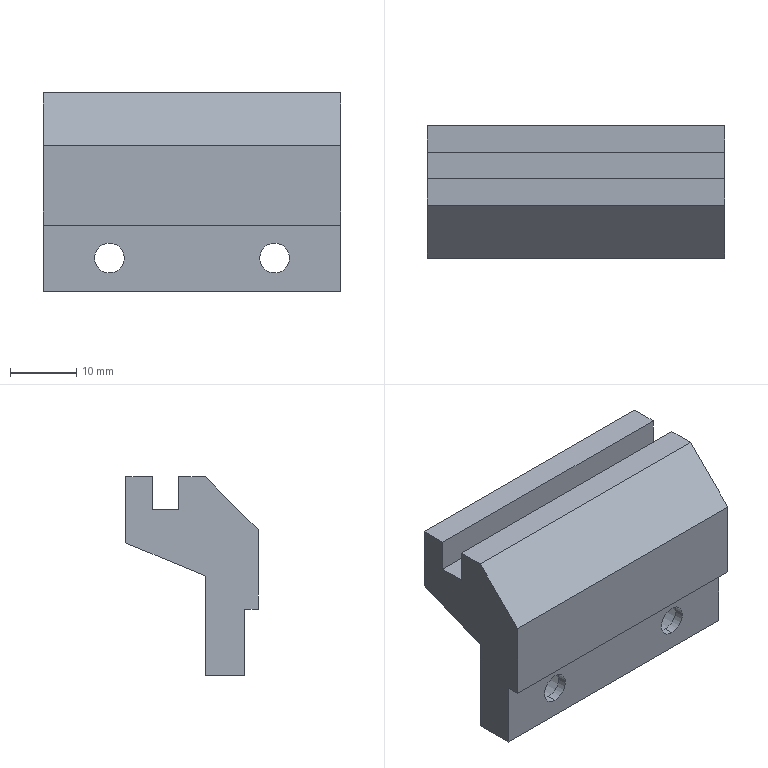Part | SolidWorks | features ICE 2, Chamfer 1, Extrusion 1, HoleWzd 1 | 1 solid | 25 faces | box 45 x 20 x 30 mm | volume 13803 mm3 | plane 17 | cylinder 8 | commonest cylinder face diameters 4.5 x4 8 x4
STEP:
#1=CARTESIAN_POINT('',(-12.5,-6.6,1.));
#2=VERTEX_POINT('',#1);
#3=CARTESIAN_POINT('',(-12.5,-6.6,9.));
#4=VERTEX_POINT('',#3);
#5=CARTESIAN_POINT('',(-12.5,-6.6,5.));
#6=DIRECTION('',(0.,1.,0.));
#7=DIRECTION('',(0.,0.,1.));
#8=AXIS2_PLACEMENT_3D('',#5,#6,#7);
#9=CIRCLE('',#8,4.);
#10=EDGE_CURVE('',#2,#4,#9,.T.);
#11=ORIENTED_EDGE('',*,*,#10,.F.);
#12=CARTESIAN_POINT('',(-12.5,-2.,1.));
#13=VERTEX_POINT('',#12);
#14=CARTESIAN_POINT('',(-12.5,-2.,1.));
#15=DIRECTION('',(0.,1.,0.));
#16=VECTOR('',#15,1000.);
#17=LINE('',#14,#16);
#18=EDGE_CURVE('',#2,#13,#17,.T.);
#19=ORIENTED_EDGE('',*,*,#18,.T.);
#20=CARTESIAN_POINT('',(-12.5,-2.,9.));
#21=VERTEX_POINT('',#20);
#22=CARTESIAN_POINT('',(-12.5,-2.,5.));
#23=DIRECTION('',(0.,1.,0.));
#24=DIRECTION('',(0.,0.,1.));
#25=AXIS2_PLACEMENT_3D('',#22,#23,#24);
#26=CIRCLE('',#25,4.);
#27=EDGE_CURVE('',#13,#21,#26,.T.);
#28=ORIENTED_EDGE('',*,*,#27,.T.);
#29=CARTESIAN_POINT('',(-12.5,-2.,9.));
#30=DIRECTION('',(0.,1.,0.));
#31=VECTOR('',#30,1000.);
#32=LINE('',#29,#31);
#33=EDGE_CURVE('',#4,#21,#32,.T.);
#34=ORIENTED_EDGE('',*,*,#33,.F.);
#35=EDGE_LOOP('',(#11,#19,#28,#34));
#36=FACE_OUTER_BOUND('',#35,.T.);
#37=CARTESIAN_POINT('',(-12.5,-2.,5.));
#38=DIRECTION('',(0.,1.,0.));
#39=DIRECTION('',(0.,0.,1.));
#40=AXIS2_PLACEMENT_3D('',#37,#38,#39);
#41=CYLINDRICAL_SURFACE('',#40,4.);
#42=ADVANCED_FACE('',(#36),#41,.F.);
#43=CARTESIAN_POINT('',(-12.5,-8.,7.25));
#44=VERTEX_POINT('',#43);
#45=CARTESIAN_POINT('',(-12.5,-8.,2.75));
#46=VERTEX_POINT('',#45);
#47=CARTESIAN_POINT('',(-12.5,-8.,5.));
#48=DIRECTION('',(0.,-1.,0.));
#49=DIRECTION('',(0.,0.,1.));
#50=AXIS2_PLACEMENT_3D('',#47,#48,#49);
#51=CIRCLE('',#50,2.25);
#52=EDGE_CURVE('',#44,#46,#51,.T.);
#53=ORIENTED_EDGE('',*,*,#52,.T.);
#54=CARTESIAN_POINT('',(-12.5,-6.6,2.75));
#55=VERTEX_POINT('',#54);
#56=CARTESIAN_POINT('',(-12.5,-2.,2.75));
#57=DIRECTION('',(0.,1.,0.));
#58=VECTOR('',#57,1000.);
#59=LINE('',#56,#58);
#60=EDGE_CURVE('',#46,#55,#59,.T.);
#61=ORIENTED_EDGE('',*,*,#60,.T.);
#62=CARTESIAN_POINT('',(-12.5,-6.6,7.25));
#63=VERTEX_POINT('',#62);
#64=CARTESIAN_POINT('',(-12.5,-6.6,5.));
#65=DIRECTION('',(0.,1.,0.));
#66=DIRECTION('',(0.,0.,1.));
#67=AXIS2_PLACEMENT_3D('',#64,#65,#66);
#68=CIRCLE('',#67,2.25);
#69=EDGE_CURVE('',#55,#63,#68,.T.);
#70=ORIENTED_EDGE('',*,*,#69,.T.);
#71=CARTESIAN_POINT('',(-12.5,-2.,7.25));
#72=DIRECTION('',(0.,1.,0.));
#73=VECTOR('',#72,1000.);
#74=LINE('',#71,#73);
#75=EDGE_CURVE('',#44,#63,#74,.T.);
#76=ORIENTED_EDGE('',*,*,#75,.F.);
#77=EDGE_LOOP('',(#53,#61,#70,#76));
#78=FACE_OUTER_BOUND('',#77,.T.);
#79=CARTESIAN_POINT('',(-12.5,-2.,5.));
#80=DIRECTION('',(0.,1.,0.));
#81=DIRECTION('',(0.,0.,1.));
#82=AXIS2_PLACEMENT_3D('',#79,#80,#81);
#83=CYLINDRICAL_SURFACE('',#82,2.25);
#84=ADVANCED_FACE('',(#78),#83,.F.);
#85=CARTESIAN_POINT('',(12.5,-6.6,1.));
#86=VERTEX_POINT('',#85);
#87=CARTESIAN_POINT('',(12.5,-6.6,9.));
#88=VERTEX_POINT('',#87);
#89=CARTESIAN_POINT('',(12.5,-6.6,5.));
#90=DIRECTION('',(0.,1.,0.));
#91=DIRECTION('',(0.,0.,1.));
#92=AXIS2_PLACEMENT_3D('',#89,#90,#91);
#93=CIRCLE('',#92,4.);
#94=EDGE_CURVE('',#86,#88,#93,.T.);
#95=ORIENTED_EDGE('',*,*,#94,.F.);
#96=CARTESIAN_POINT('',(12.5,-2.,1.));
#97=VERTEX_POINT('',#96);
#98=CARTESIAN_POINT('',(12.5,-2.,1.));
#99=DIRECTION('',(0.,1.,0.));
#100=VECTOR('',#99,1000.);
#101=LINE('',#98,#100);
#102=EDGE_CURVE('',#86,#97,#101,.T.);
#103=ORIENTED_EDGE('',*,*,#102,.T.);
#104=CARTESIAN_POINT('',(12.5,-2.,9.));
#105=VERTEX_POINT('',#104);
#106=CARTESIAN_POINT('',(12.5,-2.,5.));
#107=DIRECTION('',(0.,1.,0.));
#108=DIRECTION('',(0.,0.,1.));
#109=AXIS2_PLACEMENT_3D('',#106,#107,#108);
#110=CIRCLE('',#109,4.);
#111=EDGE_CURVE('',#97,#105,#110,.T.);
#112=ORIENTED_EDGE('',*,*,#111,.T.);
#113=CARTESIAN_POINT('',(12.5,-2.,9.));
#114=DIRECTION('',(0.,1.,0.));
#115=VECTOR('',#114,1000.);
#116=LINE('',#113,#115);
#117=EDGE_CURVE('',#88,#105,#116,.T.);
#118=ORIENTED_EDGE('',*,*,#117,.F.);
#119=EDGE_LOOP('',(#95,#103,#112,#118));
#120=FACE_OUTER_BOUND('',#119,.T.);
#121=CARTESIAN_POINT('',(12.5,-2.,5.));
#122=DIRECTION('',(0.,1.,0.));
#123=DIRECTION('',(0.,0.,1.));
#124=AXIS2_PLACEMENT_3D('',#121,#122,#123);
#125=CYLINDRICAL_SURFACE('',#124,4.);
#126=ADVANCED_FACE('',(#120),#125,.F.);
#127=CARTESIAN_POINT('',(12.5,-8.,7.25));
#128=VERTEX_POINT('',#127);
#129=CARTESIAN_POINT('',(12.5,-8.,2.75));
#130=VERTEX_POINT('',#129);
#131=CARTESIAN_POINT('',(12.5,-8.,5.));
#132=DIRECTION('',(0.,-1.,0.));
#133=DIRECTION('',(0.,0.,1.));
#134=AXIS2_PLACEMENT_3D('',#131,#132,#133);
#135=CIRCLE('',#134,2.25);
#136=EDGE_CURVE('',#128,#130,#135,.T.);
#137=ORIENTED_EDGE('',*,*,#136,.T.);
#138=CARTESIAN_POINT('',(12.5,-6.6,2.75));
#139=VERTEX_POINT('',#138);
#140=CARTESIAN_POINT('',(12.5,-2.,2.75));
#141=DIRECTION('',(0.,1.,0.));
#142=VECTOR('',#141,1000.);
#143=LINE('',#140,#142);
#144=EDGE_CURVE('',#130,#139,#143,.T.);
#145=ORIENTED_EDGE('',*,*,#144,.T.);
#146=CARTESIAN_POINT('',(12.5,-6.6,7.25));
#147=VERTEX_POINT('',#146);
#148=CARTESIAN_POINT('',(12.5,-6.6,5.));
#149=DIRECTION('',(0.,1.,0.));
#150=DIRECTION('',(0.,0.,1.));
#151=AXIS2_PLACEMENT_3D('',#148,#149,#150);
#152=CIRCLE('',#151,2.25);
#153=EDGE_CURVE('',#139,#147,#152,.T.);
#154=ORIENTED_EDGE('',*,*,#153,.T.);
#155=CARTESIAN_POINT('',(12.5,-2.,7.25));
#156=DIRECTION('',(0.,1.,0.));
#157=VECTOR('',#156,1000.);
#158=LINE('',#155,#157);
#159=EDGE_CURVE('',#128,#147,#158,.T.);
#160=ORIENTED_EDGE('',*,*,#159,.F.);
#161=EDGE_LOOP('',(#137,#145,#154,#160));
#162=FACE_OUTER_BOUND('',#161,.T.);
#163=CARTESIAN_POINT('',(12.5,-2.,5.));
#164=DIRECTION('',(0.,1.,0.));
#165=DIRECTION('',(0.,0.,1.));
#166=AXIS2_PLACEMENT_3D('',#163,#164,#165);
#167=CYLINDRICAL_SURFACE('',#166,2.25);
#168=ADVANCED_FACE('',(#162),#167,.F.);
#169=CARTESIAN_POINT('',(-22.5,2.,30.));
#170=VERTEX_POINT('',#169);
#171=CARTESIAN_POINT('',(-22.5,-2.,30.));
#172=VERTEX_POINT('',#171);
#173=CARTESIAN_POINT('',(-22.5,10.,30.));
#174=DIRECTION('',(0.,-1.,0.));
#175=VECTOR('',#174,1000.);
#176=LINE('',#173,#175);
#177=EDGE_CURVE('',#170,#172,#176,.T.);
#178=ORIENTED_EDGE('',*,*,#177,.T.);
#179=CARTESIAN_POINT('',(22.5,-2.,30.));
#180=VERTEX_POINT('',#179);
#181=CARTESIAN_POINT('',(22.5,-2.,30.));
#182=DIRECTION('',(1.,0.,0.));
#183=VECTOR('',#182,1000.);
#184=LINE('',#181,#183);
#185=EDGE_CURVE('',#172,#180,#184,.T.);
#186=ORIENTED_EDGE('',*,*,#185,.T.);
#187=CARTESIAN_POINT('',(22.5,2.,30.));
#188=VERTEX_POINT('',#187);
#189=CARTESIAN_POINT('',(22.5,10.,30.));
#190=DIRECTION('',(0.,1.,0.));
#191=VECTOR('',#190,1000.);
#192=LINE('',#189,#191);
#193=EDGE_CURVE('',#180,#188,#192,.T.);
#194=ORIENTED_EDGE('',*,*,#193,.T.);
#195=CARTESIAN_POINT('',(22.5,2.,30.));
#196=DIRECTION('',(-1.,0.,0.));
#197=VECTOR('',#196,1000.);
#198=LINE('',#195,#197);
#199=EDGE_CURVE('',#188,#170,#198,.T.);
#200=ORIENTED_EDGE('',*,*,#199,.T.);
#201=EDGE_LOOP('',(#178,#186,#194,#200));
#202=FACE_OUTER_BOUND('',#201,.T.);
#203=CARTESIAN_POINT('',(0.,0.,30.));
#204=DIRECTION('',(0.,0.,1.));
#205=DIRECTION('',(1.,0.,0.));
#206=AXIS2_PLACEMENT_3D('',#203,#204,#205);
#207=PLANE('',#206);
#208=ADVANCED_FACE('',(#202),#207,.T.);
#209=CARTESIAN_POINT('',(22.5,-10.,10.));
#210=VERTEX_POINT('',#209);
#211=CARTESIAN_POINT('',(22.5,-8.,10.));
#212=VERTEX_POINT('',#211);
#213=CARTESIAN_POINT('',(22.5,-8.,10.));
#214=DIRECTION('',(0.,1.,0.));
#215=VECTOR('',#214,1000.);
#216=LINE('',#213,#215);
#217=EDGE_CURVE('',#210,#212,#216,.T.);
#218=ORIENTED_EDGE('',*,*,#217,.T.);
#219=CARTESIAN_POINT('',(22.5,-8.,0.));
#220=VERTEX_POINT('',#219);
#221=CARTESIAN_POINT('',(22.5,-8.,0.));
#222=DIRECTION('',(0.,0.,-1.));
#223=VECTOR('',#222,1000.);
#224=LINE('',#221,#223);
#225=EDGE_CURVE('',#212,#220,#224,.T.);
#226=ORIENTED_EDGE('',*,*,#225,.T.);
#227=CARTESIAN_POINT('',(22.5,-2.,0.));
#228=VERTEX_POINT('',#227);
#229=CARTESIAN_POINT('',(22.5,10.,0.));
#230=DIRECTION('',(0.,1.,0.));
#231=VECTOR('',#230,1000.);
#232=LINE('',#229,#231);
#233=EDGE_CURVE('',#220,#228,#232,.T.);
#234=ORIENTED_EDGE('',*,*,#233,.T.);
#235=CARTESIAN_POINT('',(22.5,-2.,15.));
#236=VERTEX_POINT('',#235);
#237=CARTESIAN_POINT('',(22.5,-2.,0.));
#238=DIRECTION('',(0.,0.,1.));
#239=VECTOR('',#238,1000.);
#240=LINE('',#237,#239);
#241=EDGE_CURVE('',#228,#236,#240,.T.);
#242=ORIENTED_EDGE('',*,*,#241,.T.);
#243=CARTESIAN_POINT('',(22.5,10.,20.));
#244=VERTEX_POINT('',#243);
#245=CARTESIAN_POINT('',(22.5,-2.,15.));
#246=DIRECTION('',(0.,0.9231,0.3846));
#247=VECTOR('',#246,1000.);
#248=LINE('',#245,#247);
#249=EDGE_CURVE('',#236,#244,#248,.T.);
#250=ORIENTED_EDGE('',*,*,#249,.T.);
#251=CARTESIAN_POINT('',(22.5,10.,30.));
#252=VERTEX_POINT('',#251);
#253=CARTESIAN_POINT('',(22.5,10.,30.));
#254=DIRECTION('',(0.,0.,-1.));
#255=VECTOR('',#254,1000.);
#256=LINE('',#253,#255);
#257=EDGE_CURVE('',#252,#244,#256,.T.);
#258=ORIENTED_EDGE('',*,*,#257,.F.);
#259=CARTESIAN_POINT('',(22.5,6.,30.));
#260=VERTEX_POINT('',#259);
#261=CARTESIAN_POINT('',(22.5,10.,30.));
#262=DIRECTION('',(0.,1.,0.));
#263=VECTOR('',#262,1000.);
#264=LINE('',#261,#263);
#265=EDGE_CURVE('',#260,#252,#264,.T.);
#266=ORIENTED_EDGE('',*,*,#265,.F.);
#267=CARTESIAN_POINT('',(22.5,6.,25.));
#268=VERTEX_POINT('',#267);
#269=CARTESIAN_POINT('',(22.5,6.,30.));
#270=DIRECTION('',(0.,0.,-1.));
#271=VECTOR('',#270,1000.);
#272=LINE('',#269,#271);
#273=EDGE_CURVE('',#260,#268,#272,.T.);
#274=ORIENTED_EDGE('',*,*,#273,.T.);
#275=CARTESIAN_POINT('',(22.5,2.,25.));
#276=VERTEX_POINT('',#275);
#277=CARTESIAN_POINT('',(22.5,6.,25.));
#278=DIRECTION('',(0.,-1.,0.));
#279=VECTOR('',#278,1000.);
#280=LINE('',#277,#279);
#281=EDGE_CURVE('',#268,#276,#280,.T.);
#282=ORIENTED_EDGE('',*,*,#281,.T.);
#283=CARTESIAN_POINT('',(22.5,2.,30.));
#284=DIRECTION('',(0.,0.,1.));
#285=VECTOR('',#284,1000.);
#286=LINE('',#283,#285);
#287=EDGE_CURVE('',#276,#188,#286,.T.);
#288=ORIENTED_EDGE('',*,*,#287,.T.);
#289=ORIENTED_EDGE('',*,*,#193,.F.);
#290=CARTESIAN_POINT('',(22.5,-10.,22.));
#291=VERTEX_POINT('',#290);
#292=CARTESIAN_POINT('',(22.5,-2.,30.));
#293=DIRECTION('',(0.,-0.7071,-0.7071));
#294=VECTOR('',#293,1000.);
#295=LINE('',#292,#294);
#296=EDGE_CURVE('',#180,#291,#295,.T.);
#297=ORIENTED_EDGE('',*,*,#296,.T.);
#298=CARTESIAN_POINT('',(22.5,-10.,30.));
#299=DIRECTION('',(0.,0.,-1.));
#300=VECTOR('',#299,1000.);
#301=LINE('',#298,#300);
#302=EDGE_CURVE('',#291,#210,#301,.T.);
#303=ORIENTED_EDGE('',*,*,#302,.T.);
#304=EDGE_LOOP('',(#218,#226,#234,#242,#250,#258,#266,#274,#282,#288,#289,#297,#303));
#305=FACE_OUTER_BOUND('',#304,.T.);
#306=CARTESIAN_POINT('',(22.5,10.,30.));
#307=DIRECTION('',(-1.,0.,0.));
#308=DIRECTION('',(0.,0.,1.));
#309=AXIS2_PLACEMENT_3D('',#306,#307,#308);
#310=PLANE('',#309);
#311=ADVANCED_FACE('',(#305),#310,.F.);
#312=ORIENTED_EDGE('',*,*,#257,.T.);
#313=CARTESIAN_POINT('',(-22.5,10.,20.));
#314=VERTEX_POINT('',#313);
#315=CARTESIAN_POINT('',(22.5,10.,20.));
#316=DIRECTION('',(-1.,0.,0.));
#317=VECTOR('',#316,1000.);
#318=LINE('',#315,#317);
#319=EDGE_CURVE('',#244,#314,#318,.T.);
#320=ORIENTED_EDGE('',*,*,#319,.T.);
#321=CARTESIAN_POINT('',(-22.5,10.,30.));
#322=VERTEX_POINT('',#321);
#323=CARTESIAN_POINT('',(-22.5,10.,30.));
#324=DIRECTION('',(0.,0.,-1.));
#325=VECTOR('',#324,1000.);
#326=LINE('',#323,#325);
#327=EDGE_CURVE('',#322,#314,#326,.T.);
#328=ORIENTED_EDGE('',*,*,#327,.F.);
#329=CARTESIAN_POINT('',(-22.5,10.,30.));
#330=DIRECTION('',(-1.,0.,0.));
#331=VECTOR('',#330,1000.);
#332=LINE('',#329,#331);
#333=EDGE_CURVE('',#252,#322,#332,.T.);
#334=ORIENTED_EDGE('',*,*,#333,.F.);
#335=EDGE_LOOP('',(#312,#320,#328,#334));
#336=FACE_OUTER_BOUND('',#335,.T.);
#337=CARTESIAN_POINT('',(-22.5,10.,30.));
#338=DIRECTION('',(0.,-1.,0.));
#339=DIRECTION('',(0.,0.,-1.));
#340=AXIS2_PLACEMENT_3D('',#337,#338,#339);
#341=PLANE('',#340);
#342=ADVANCED_FACE('',(#336),#341,.F.);
#343=CARTESIAN_POINT('',(-22.5,-2.,0.));
#344=VERTEX_POINT('',#343);
#345=CARTESIAN_POINT('',(-22.5,-8.,0.));
#346=VERTEX_POINT('',#345);
#347=CARTESIAN_POINT('',(-22.5,10.,0.));
#348=DIRECTION('',(0.,-1.,0.));
#349=VECTOR('',#348,1000.);
#350=LINE('',#347,#349);
#351=EDGE_CURVE('',#344,#346,#350,.T.);
#352=ORIENTED_EDGE('',*,*,#351,.T.);
#353=CARTESIAN_POINT('',(-22.5,-8.,10.));
#354=VERTEX_POINT('',#353);
#355=CARTESIAN_POINT('',(-22.5,-8.,30.));
#356=DIRECTION('',(0.,0.,1.));
#357=VECTOR('',#356,1000.);
#358=LINE('',#355,#357);
#359=EDGE_CURVE('',#346,#354,#358,.T.);
#360=ORIENTED_EDGE('',*,*,#359,.T.);
#361=CARTESIAN_POINT('',(-22.5,-10.,10.));
#362=VERTEX_POINT('',#361);
#363=CARTESIAN_POINT('',(-22.5,10.,10.));
#364=DIRECTION('',(0.,-1.,0.));
#365=VECTOR('',#364,1000.);
#366=LINE('',#363,#365);
#367=EDGE_CURVE('',#354,#362,#366,.T.);
#368=ORIENTED_EDGE('',*,*,#367,.T.);
#369=CARTESIAN_POINT('',(-22.5,-10.,22.));
#370=VERTEX_POINT('',#369);
#371=CARTESIAN_POINT('',(-22.5,-10.,30.));
#372=DIRECTION('',(0.,0.,-1.));
#373=VECTOR('',#372,1000.);
#374=LINE('',#371,#373);
#375=EDGE_CURVE('',#370,#362,#374,.T.);
#376=ORIENTED_EDGE('',*,*,#375,.F.);
#377=CARTESIAN_POINT('',(-22.5,-2.,30.));
#378=DIRECTION('',(0.,0.7071,0.7071));
#379=VECTOR('',#378,1000.);
#380=LINE('',#377,#379);
#381=EDGE_CURVE('',#370,#172,#380,.T.);
#382=ORIENTED_EDGE('',*,*,#381,.T.);
#383=ORIENTED_EDGE('',*,*,#177,.F.);
#384=CARTESIAN_POINT('',(-22.5,2.,25.));
#385=VERTEX_POINT('',#384);
#386=CARTESIAN_POINT('',(-22.5,2.,30.));
#387=DIRECTION('',(0.,0.,-1.));
#388=VECTOR('',#387,1000.);
#389=LINE('',#386,#388);
#390=EDGE_CURVE('',#170,#385,#389,.T.);
#391=ORIENTED_EDGE('',*,*,#390,.T.);
#392=CARTESIAN_POINT('',(-22.5,6.,25.));
#393=VERTEX_POINT('',#392);
#394=CARTESIAN_POINT('',(-22.5,10.,25.));
#395=DIRECTION('',(0.,1.,0.));
#396=VECTOR('',#395,1000.);
#397=LINE('',#394,#396);
#398=EDGE_CURVE('',#385,#393,#397,.T.);
#399=ORIENTED_EDGE('',*,*,#398,.T.);
#400=CARTESIAN_POINT('',(-22.5,6.,30.));
#401=VERTEX_POINT('',#400);
#402=CARTESIAN_POINT('',(-22.5,6.,30.));
#403=DIRECTION('',(0.,0.,1.));
#404=VECTOR('',#403,1000.);
#405=LINE('',#402,#404);
#406=EDGE_CURVE('',#393,#401,#405,.T.);
#407=ORIENTED_EDGE('',*,*,#406,.T.);
#408=CARTESIAN_POINT('',(-22.5,10.,30.));
#409=DIRECTION('',(0.,-1.,0.));
#410=VECTOR('',#409,1000.);
#411=LINE('',#408,#410);
#412=EDGE_CURVE('',#322,#401,#411,.T.);
#413=ORIENTED_EDGE('',*,*,#412,.F.);
#414=ORIENTED_EDGE('',*,*,#327,.T.);
#415=CARTESIAN_POINT('',(-22.5,-2.,15.));
#416=VERTEX_POINT('',#415);
#417=CARTESIAN_POINT('',(-22.5,13.55,21.479));
#418=DIRECTION('',(0.,-0.9231,-0.3846));
#419=VECTOR('',#418,1000.);
#420=LINE('',#417,#419);
#421=EDGE_CURVE('',#314,#416,#420,.T.);
#422=ORIENTED_EDGE('',*,*,#421,.T.);
#423=CARTESIAN_POINT('',(-22.5,-2.,30.));
#424=DIRECTION('',(0.,0.,-1.));
#425=VECTOR('',#424,1000.);
#426=LINE('',#423,#425);
#427=EDGE_CURVE('',#416,#344,#426,.T.);
#428=ORIENTED_EDGE('',*,*,#427,.T.);
#429=EDGE_LOOP('',(#352,#360,#368,#376,#382,#383,#391,#399,#407,#413,#414,#422,#428));
#430=FACE_OUTER_BOUND('',#429,.T.);
#431=CARTESIAN_POINT('',(-22.5,10.,30.));
#432=DIRECTION('',(1.,0.,0.));
#433=DIRECTION('',(0.,0.,-1.));
#434=AXIS2_PLACEMENT_3D('',#431,#432,#433);
#435=PLANE('',#434);
#436=ADVANCED_FACE('',(#430),#435,.F.);
#437=ORIENTED_EDGE('',*,*,#375,.T.);
#438=CARTESIAN_POINT('',(22.5,-10.,10.));
#439=DIRECTION('',(-1.,0.,0.));
#440=VECTOR('',#439,1000.);
#441=LINE('',#438,#440);
#442=EDGE_CURVE('',#210,#362,#441,.T.);
#443=ORIENTED_EDGE('',*,*,#442,.F.);
#444=ORIENTED_EDGE('',*,*,#302,.F.);
#445=CARTESIAN_POINT('',(-22.5,-10.,22.));
#446=DIRECTION('',(-1.,0.,0.));
#447=VECTOR('',#446,1000.);
#448=LINE('',#445,#447);
#449=EDGE_CURVE('',#291,#370,#448,.T.);
#450=ORIENTED_EDGE('',*,*,#449,.T.);
#451=EDGE_LOOP('',(#437,#443,#444,#450));
#452=FACE_OUTER_BOUND('',#451,.T.);
#453=CARTESIAN_POINT('',(-22.5,-10.,30.));
#454=DIRECTION('',(0.,1.,0.));
#455=DIRECTION('',(0.,0.,1.));
#456=AXIS2_PLACEMENT_3D('',#453,#454,#455);
#457=PLANE('',#456);
#458=ADVANCED_FACE('',(#452),#457,.F.);
#459=CARTESIAN_POINT('',(22.5,6.,30.));
#460=DIRECTION('',(-1.,0.,0.));
#461=VECTOR('',#460,1000.);
#462=LINE('',#459,#461);
#463=EDGE_CURVE('',#260,#401,#462,.T.);
#464=ORIENTED_EDGE('',*,*,#463,.F.);
#465=ORIENTED_EDGE('',*,*,#265,.T.);
#466=ORIENTED_EDGE('',*,*,#333,.T.);
#467=ORIENTED_EDGE('',*,*,#412,.T.);
#468=EDGE_LOOP('',(#464,#465,#466,#467));
#469=FACE_OUTER_BOUND('',#468,.T.);
#470=CARTESIAN_POINT('',(0.,0.,30.));
#471=DIRECTION('',(0.,0.,1.));
#472=DIRECTION('',(1.,0.,0.));
#473=AXIS2_PLACEMENT_3D('',#470,#471,#472);
#474=PLANE('',#473);
#475=ADVANCED_FACE('',(#469),#474,.T.);
#476=ORIENTED_EDGE('',*,*,#233,.F.);
#477=CARTESIAN_POINT('',(22.5,-8.,0.));
#478=DIRECTION('',(-1.,0.,0.));
#479=VECTOR('',#478,1000.);
#480=LINE('',#477,#479);
#481=EDGE_CURVE('',#220,#346,#480,.T.);
#482=ORIENTED_EDGE('',*,*,#481,.T.);
#483=ORIENTED_EDGE('',*,*,#351,.F.);
#484=CARTESIAN_POINT('',(22.5,-2.,0.));
#485=DIRECTION('',(-1.,0.,0.));
#486=VECTOR('',#485,1000.);
#487=LINE('',#484,#486);
#488=EDGE_CURVE('',#228,#344,#487,.T.);
#489=ORIENTED_EDGE('',*,*,#488,.F.);
#490=EDGE_LOOP('',(#476,#482,#483,#489));
#491=FACE_OUTER_BOUND('',#490,.T.);
#492=CARTESIAN_POINT('',(0.,0.,0.));
#493=DIRECTION('',(0.,0.,1.));
#494=DIRECTION('',(1.,0.,0.));
#495=AXIS2_PLACEMENT_3D('',#492,#493,#494);
#496=PLANE('',#495);
#497=ADVANCED_FACE('',(#491),#496,.F.);
#498=ORIENTED_EDGE('',*,*,#319,.F.);
#499=ORIENTED_EDGE('',*,*,#249,.F.);
#500=CARTESIAN_POINT('',(22.5,-2.,15.));
#501=DIRECTION('',(-1.,0.,0.));
#502=VECTOR('',#501,1000.);
#503=LINE('',#500,#502);
#504=EDGE_CURVE('',#236,#416,#503,.T.);
#505=ORIENTED_EDGE('',*,*,#504,.T.);
#506=ORIENTED_EDGE('',*,*,#421,.F.);
#507=EDGE_LOOP('',(#498,#499,#505,#506));
#508=FACE_OUTER_BOUND('',#507,.T.);
#509=CARTESIAN_POINT('',(22.5,-2.,15.));
#510=DIRECTION('',(0.,-0.3846,0.9231));
#511=DIRECTION('',(0.,-0.9231,-0.3846));
#512=AXIS2_PLACEMENT_3D('',#509,#510,#511);
#513=PLANE('',#512);
#514=ADVANCED_FACE('',(#508),#513,.F.);
#515=CARTESIAN_POINT('',(-12.5,-2.,5.));
#516=DIRECTION('',(0.,1.,0.));
#517=DIRECTION('',(0.,0.,1.));
#518=AXIS2_PLACEMENT_3D('',#515,#516,#517);
#519=CIRCLE('',#518,4.);
#520=EDGE_CURVE('',#21,#13,#519,.T.);
#521=ORIENTED_EDGE('',*,*,#520,.F.);
#522=ORIENTED_EDGE('',*,*,#27,.F.);
#523=EDGE_LOOP('',(#521,#522));
#524=FACE_BOUND('',#523,.T.);
#525=CARTESIAN_POINT('',(12.5,-2.,5.));
#526=DIRECTION('',(0.,1.,0.));
#527=DIRECTION('',(0.,0.,1.));
#528=AXIS2_PLACEMENT_3D('',#525,#526,#527);
#529=CIRCLE('',#528,4.);
#530=EDGE_CURVE('',#105,#97,#529,.T.);
#531=ORIENTED_EDGE('',*,*,#530,.F.);
#532=ORIENTED_EDGE('',*,*,#111,.F.);
#533=EDGE_LOOP('',(#531,#532));
#534=FACE_BOUND('',#533,.T.);
#535=ORIENTED_EDGE('',*,*,#504,.F.);
#536=ORIENTED_EDGE('',*,*,#241,.F.);
#537=ORIENTED_EDGE('',*,*,#488,.T.);
#538=ORIENTED_EDGE('',*,*,#427,.F.);
#539=EDGE_LOOP('',(#535,#536,#537,#538));
#540=FACE_OUTER_BOUND('',#539,.T.);
#541=CARTESIAN_POINT('',(22.5,-2.,0.));
#542=DIRECTION('',(0.,-1.,0.));
#543=DIRECTION('',(0.,0.,-1.));
#544=AXIS2_PLACEMENT_3D('',#541,#542,#543);
#545=PLANE('',#544);
#546=ADVANCED_FACE('',(#524,#534,#540),#545,.F.);
#547=CARTESIAN_POINT('',(22.5,2.,25.));
#548=DIRECTION('',(-1.,0.,0.));
#549=VECTOR('',#548,1000.);
#550=LINE('',#547,#549);
#551=EDGE_CURVE('',#276,#385,#550,.T.);
#552=ORIENTED_EDGE('',*,*,#551,.F.);
#553=ORIENTED_EDGE('',*,*,#281,.F.);
#554=CARTESIAN_POINT('',(22.5,6.,25.));
#555=DIRECTION('',(-1.,0.,0.));
#556=VECTOR('',#555,1000.);
#557=LINE('',#554,#556);
#558=EDGE_CURVE('',#268,#393,#557,.T.);
#559=ORIENTED_EDGE('',*,*,#558,.T.);
#560=ORIENTED_EDGE('',*,*,#398,.F.);
#561=EDGE_LOOP('',(#552,#553,#559,#560));
#562=FACE_OUTER_BOUND('',#561,.T.);
#563=CARTESIAN_POINT('',(22.5,6.,25.));
#564=DIRECTION('',(0.,0.,-1.));
#565=DIRECTION('',(-1.,0.,0.));
#566=AXIS2_PLACEMENT_3D('',#563,#564,#565);
#567=PLANE('',#566);
#568=ADVANCED_FACE('',(#562),#567,.F.);
#569=ORIENTED_EDGE('',*,*,#199,.F.);
#570=ORIENTED_EDGE('',*,*,#287,.F.);
#571=ORIENTED_EDGE('',*,*,#551,.T.);
#572=ORIENTED_EDGE('',*,*,#390,.F.);
#573=EDGE_LOOP('',(#569,#570,#571,#572));
#574=FACE_OUTER_BOUND('',#573,.T.);
#575=CARTESIAN_POINT('',(22.5,2.,30.));
#576=DIRECTION('',(0.,-1.,0.));
#577=DIRECTION('',(0.,0.,-1.));
#578=AXIS2_PLACEMENT_3D('',#575,#576,#577);
#579=PLANE('',#578);
#580=ADVANCED_FACE('',(#574),#579,.F.);
#581=ORIENTED_EDGE('',*,*,#558,.F.);
#582=ORIENTED_EDGE('',*,*,#273,.F.);
#583=ORIENTED_EDGE('',*,*,#463,.T.);
#584=ORIENTED_EDGE('',*,*,#406,.F.);
#585=EDGE_LOOP('',(#581,#582,#583,#584));
#586=FACE_OUTER_BOUND('',#585,.T.);
#587=CARTESIAN_POINT('',(22.5,6.,30.));
#588=DIRECTION('',(0.,1.,0.));
#589=DIRECTION('',(0.,0.,1.));
#590=AXIS2_PLACEMENT_3D('',#587,#588,#589);
#591=PLANE('',#590);
#592=ADVANCED_FACE('',(#586),#591,.F.);
#593=ORIENTED_EDGE('',*,*,#381,.F.);
#594=ORIENTED_EDGE('',*,*,#449,.F.);
#595=ORIENTED_EDGE('',*,*,#296,.F.);
#596=ORIENTED_EDGE('',*,*,#185,.F.);
#597=EDGE_LOOP('',(#593,#594,#595,#596));
#598=FACE_OUTER_BOUND('',#597,.T.);
#599=CARTESIAN_POINT('',(0.,-2.,30.));
#600=DIRECTION('',(0.,-0.7071,0.7071));
#601=DIRECTION('',(-1.,0.,0.));
#602=AXIS2_PLACEMENT_3D('',#599,#600,#601);
#603=PLANE('',#602);
#604=ADVANCED_FACE('',(#598),#603,.T.);
#605=ORIENTED_EDGE('',*,*,#144,.F.);
#606=CARTESIAN_POINT('',(12.5,-8.,5.));
#607=DIRECTION('',(0.,-1.,0.));
#608=DIRECTION('',(0.,0.,1.));
#609=AXIS2_PLACEMENT_3D('',#606,#607,#608);
#610=CIRCLE('',#609,2.25);
#611=EDGE_CURVE('',#130,#128,#610,.T.);
#612=ORIENTED_EDGE('',*,*,#611,.T.);
#613=ORIENTED_EDGE('',*,*,#159,.T.);
#614=CARTESIAN_POINT('',(12.5,-6.6,5.));
#615=DIRECTION('',(0.,1.,0.));
#616=DIRECTION('',(0.,0.,1.));
#617=AXIS2_PLACEMENT_3D('',#614,#615,#616);
#618=CIRCLE('',#617,2.25);
#619=EDGE_CURVE('',#147,#139,#618,.T.);
#620=ORIENTED_EDGE('',*,*,#619,.T.);
#621=EDGE_LOOP('',(#605,#612,#613,#620));
#622=FACE_OUTER_BOUND('',#621,.T.);
#623=CARTESIAN_POINT('',(12.5,-2.,5.));
#624=DIRECTION('',(0.,1.,0.));
#625=DIRECTION('',(0.,0.,1.));
#626=AXIS2_PLACEMENT_3D('',#623,#624,#625);
#627=CYLINDRICAL_SURFACE('',#626,2.25);
#628=ADVANCED_FACE('',(#622),#627,.F.);
#629=ORIENTED_EDGE('',*,*,#619,.F.);
#630=ORIENTED_EDGE('',*,*,#153,.F.);
#631=EDGE_LOOP('',(#629,#630));
#632=FACE_BOUND('',#631,.T.);
#633=CARTESIAN_POINT('',(12.5,-6.6,5.));
#634=DIRECTION('',(0.,1.,0.));
#635=DIRECTION('',(0.,0.,1.));
#636=AXIS2_PLACEMENT_3D('',#633,#634,#635);
#637=CIRCLE('',#636,4.);
#638=EDGE_CURVE('',#88,#86,#637,.T.);
#639=ORIENTED_EDGE('',*,*,#638,.T.);
#640=ORIENTED_EDGE('',*,*,#94,.T.);
#641=EDGE_LOOP('',(#639,#640));
#642=FACE_OUTER_BOUND('',#641,.T.);
#643=CARTESIAN_POINT('',(14.75,-6.6,5.));
#644=DIRECTION('',(0.,-1.,0.));
#645=DIRECTION('',(0.,0.,-1.));
#646=AXIS2_PLACEMENT_3D('',#643,#644,#645);
#647=PLANE('',#646);
#648=ADVANCED_FACE('',(#632,#642),#647,.F.);
#649=ORIENTED_EDGE('',*,*,#102,.F.);
#650=ORIENTED_EDGE('',*,*,#638,.F.);
#651=ORIENTED_EDGE('',*,*,#117,.T.);
#652=ORIENTED_EDGE('',*,*,#530,.T.);
#653=EDGE_LOOP('',(#649,#650,#651,#652));
#654=FACE_OUTER_BOUND('',#653,.T.);
#655=CARTESIAN_POINT('',(12.5,-2.,5.));
#656=DIRECTION('',(0.,1.,0.));
#657=DIRECTION('',(0.,0.,1.));
#658=AXIS2_PLACEMENT_3D('',#655,#656,#657);
#659=CYLINDRICAL_SURFACE('',#658,4.);
#660=ADVANCED_FACE('',(#654),#659,.F.);
#661=ORIENTED_EDGE('',*,*,#60,.F.);
#662=CARTESIAN_POINT('',(-12.5,-8.,5.));
#663=DIRECTION('',(0.,-1.,0.));
#664=DIRECTION('',(0.,0.,1.));
#665=AXIS2_PLACEMENT_3D('',#662,#663,#664);
#666=CIRCLE('',#665,2.25);
#667=EDGE_CURVE('',#46,#44,#666,.T.);
#668=ORIENTED_EDGE('',*,*,#667,.T.);
#669=ORIENTED_EDGE('',*,*,#75,.T.);
#670=CARTESIAN_POINT('',(-12.5,-6.6,5.));
#671=DIRECTION('',(0.,1.,0.));
#672=DIRECTION('',(0.,0.,1.));
#673=AXIS2_PLACEMENT_3D('',#670,#671,#672);
#674=CIRCLE('',#673,2.25);
#675=EDGE_CURVE('',#63,#55,#674,.T.);
#676=ORIENTED_EDGE('',*,*,#675,.T.);
#677=EDGE_LOOP('',(#661,#668,#669,#676));
#678=FACE_OUTER_BOUND('',#677,.T.);
#679=CARTESIAN_POINT('',(-12.5,-2.,5.));
#680=DIRECTION('',(0.,1.,0.));
#681=DIRECTION('',(0.,0.,1.));
#682=AXIS2_PLACEMENT_3D('',#679,#680,#681);
#683=CYLINDRICAL_SURFACE('',#682,2.25);
#684=ADVANCED_FACE('',(#678),#683,.F.);
#685=ORIENTED_EDGE('',*,*,#675,.F.);
#686=ORIENTED_EDGE('',*,*,#69,.F.);
#687=EDGE_LOOP('',(#685,#686));
#688=FACE_BOUND('',#687,.T.);
#689=CARTESIAN_POINT('',(-12.5,-6.6,5.));
#690=DIRECTION('',(0.,1.,0.));
#691=DIRECTION('',(0.,0.,1.));
#692=AXIS2_PLACEMENT_3D('',#689,#690,#691);
#693=CIRCLE('',#692,4.);
#694=EDGE_CURVE('',#4,#2,#693,.T.);
#695=ORIENTED_EDGE('',*,*,#694,.T.);
#696=ORIENTED_EDGE('',*,*,#10,.T.);
#697=EDGE_LOOP('',(#695,#696));
#698=FACE_OUTER_BOUND('',#697,.T.);
#699=CARTESIAN_POINT('',(-10.25,-6.6,5.));
#700=DIRECTION('',(0.,-1.,0.));
#701=DIRECTION('',(0.,0.,-1.));
#702=AXIS2_PLACEMENT_3D('',#699,#700,#701);
#703=PLANE('',#702);
#704=ADVANCED_FACE('',(#688,#698),#703,.F.);
#705=ORIENTED_EDGE('',*,*,#18,.F.);
#706=ORIENTED_EDGE('',*,*,#694,.F.);
#707=ORIENTED_EDGE('',*,*,#33,.T.);
#708=ORIENTED_EDGE('',*,*,#520,.T.);
#709=EDGE_LOOP('',(#705,#706,#707,#708));
#710=FACE_OUTER_BOUND('',#709,.T.);
#711=CARTESIAN_POINT('',(-12.5,-2.,5.));
#712=DIRECTION('',(0.,1.,0.));
#713=DIRECTION('',(0.,0.,1.));
#714=AXIS2_PLACEMENT_3D('',#711,#712,#713);
#715=CYLINDRICAL_SURFACE('',#714,4.);
#716=ADVANCED_FACE('',(#710),#715,.F.);
#717=CARTESIAN_POINT('',(22.5,-8.,10.));
#718=DIRECTION('',(-1.,0.,0.));
#719=VECTOR('',#718,1000.);
#720=LINE('',#717,#719);
#721=EDGE_CURVE('',#212,#354,#720,.T.);
#722=ORIENTED_EDGE('',*,*,#721,.F.);
#723=ORIENTED_EDGE('',*,*,#217,.F.);
#724=ORIENTED_EDGE('',*,*,#442,.T.);
#725=ORIENTED_EDGE('',*,*,#367,.F.);
#726=EDGE_LOOP('',(#722,#723,#724,#725));
#727=FACE_OUTER_BOUND('',#726,.T.);
#728=CARTESIAN_POINT('',(22.5,-8.,10.));
#729=DIRECTION('',(0.,0.,1.));
#730=DIRECTION('',(1.,0.,0.));
#731=AXIS2_PLACEMENT_3D('',#728,#729,#730);
#732=PLANE('',#731);
#733=ADVANCED_FACE('',(#727),#732,.F.);
#734=ORIENTED_EDGE('',*,*,#52,.F.);
#735=ORIENTED_EDGE('',*,*,#667,.F.);
#736=EDGE_LOOP('',(#734,#735));
#737=FACE_BOUND('',#736,.T.);
#738=ORIENTED_EDGE('',*,*,#136,.F.);
#739=ORIENTED_EDGE('',*,*,#611,.F.);
#740=EDGE_LOOP('',(#738,#739));
#741=FACE_BOUND('',#740,.T.);
#742=ORIENTED_EDGE('',*,*,#481,.F.);
#743=ORIENTED_EDGE('',*,*,#225,.F.);
#744=ORIENTED_EDGE('',*,*,#721,.T.);
#745=ORIENTED_EDGE('',*,*,#359,.F.);
#746=EDGE_LOOP('',(#742,#743,#744,#745));
#747=FACE_OUTER_BOUND('',#746,.T.);
#748=CARTESIAN_POINT('',(22.5,-8.,0.));
#749=DIRECTION('',(0.,1.,0.));
#750=DIRECTION('',(0.,0.,1.));
#751=AXIS2_PLACEMENT_3D('',#748,#749,#750);
#752=PLANE('',#751);
#753=ADVANCED_FACE('',(#737,#741,#747),#752,.F.);
#754=CLOSED_SHELL('',(#42,#84,#126,#168,#208,#311,#342,#436,#458,#475,#497,#514,#546,#568,#580,#592,#604,#628,#648,#660,#684,#704,#716,#733,#753));
#755=MANIFOLD_SOLID_BREP('',#754);
#756=CARTESIAN_POINT('',(0.,0.,0.));
#757=DIRECTION('',(0.,0.,1.));
#758=DIRECTION('',(1.,0.,0.));
#759=AXIS2_PLACEMENT_3D('',#756,#757,#758);
#760=(LENGTH_UNIT()NAMED_UNIT(*)SI_UNIT(.MILLI.,.METRE.));
#761=UNCERTAINTY_MEASURE_WITH_UNIT(LENGTH_MEASURE(0.00001),#760,'','');
#762=(NAMED_UNIT(*)PLANE_ANGLE_UNIT()SI_UNIT($,.RADIAN.));
#763=(NAMED_UNIT(*)SI_UNIT($,.STERADIAN.)SOLID_ANGLE_UNIT());
#764=(GEOMETRIC_REPRESENTATION_CONTEXT(3)GLOBAL_UNCERTAINTY_ASSIGNED_CONTEXT((#761))GLOBAL_UNIT_ASSIGNED_CONTEXT((#760,#762,#763))REPRESENTATION_CONTEXT('',''));
#765=ADVANCED_BREP_SHAPE_REPRESENTATION('',(#755,#759),#764);